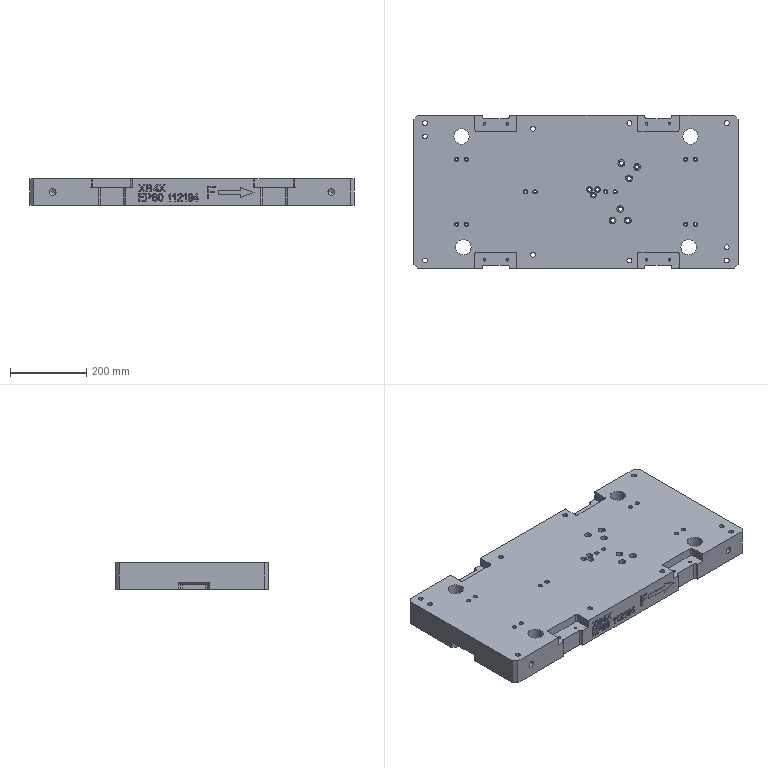Part | CATIA | 17 solids | 1306 faces | box 850 x 401 x 70 mm | volume 21718763 mm3 | plane 848 | cylinder 356 | cone 102 | commonest cylinder face diameters 10 x74 6.8 x64 20 x48 11 x36 7 x24 40 x20